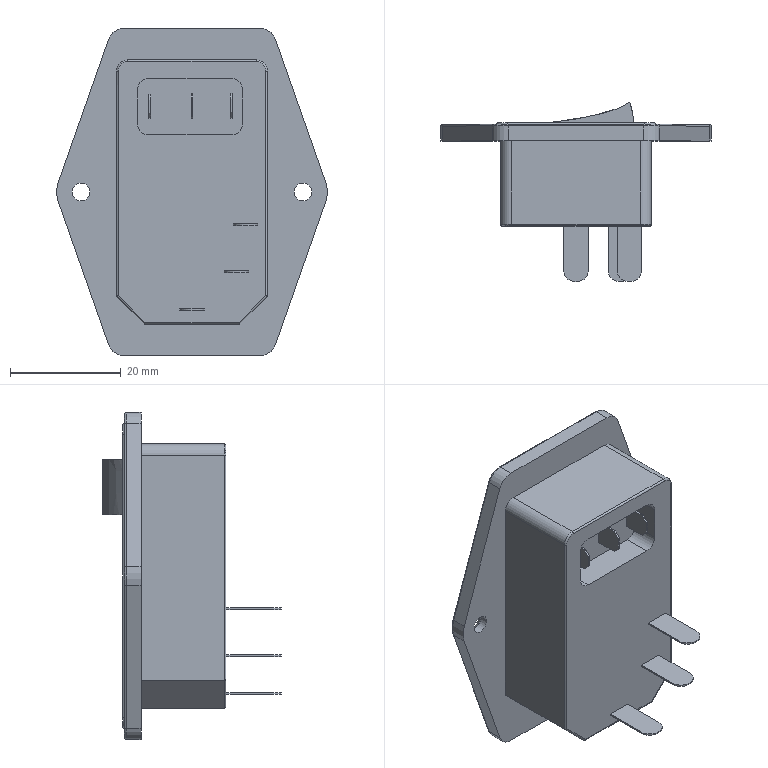Part | STEP file | Power supply socket base 1 | 1 solid | 179 faces | box 48.802 x 32.25 x 59 mm | volume 19830 mm3 | plane 101 | cylinder 54 | torus 18 | cone 4 | other 2 | commonest cylinder face diameters 0.6 x22 4 x12 6 x8 1 x4 3.2 x4 2 x2